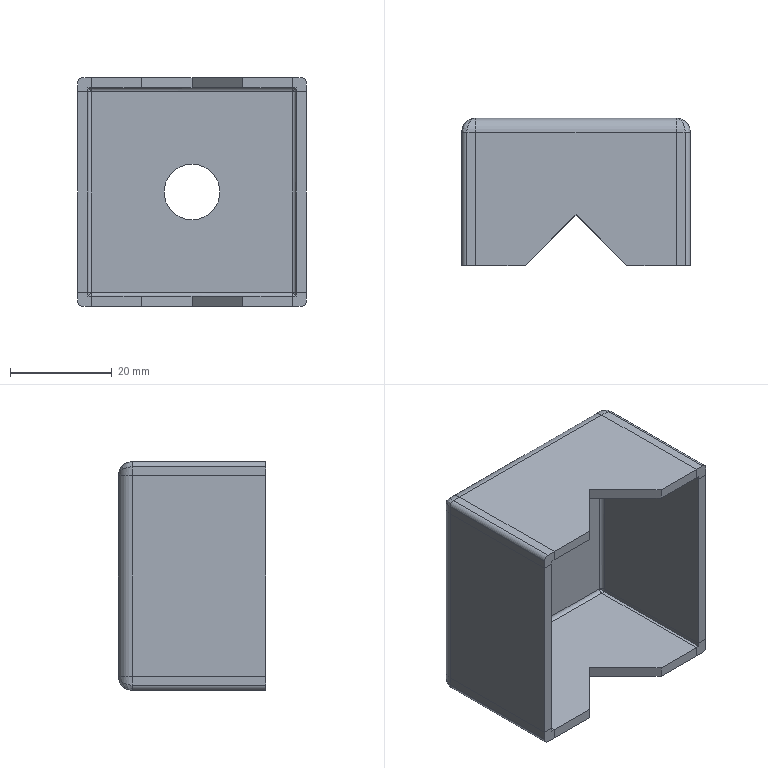Part | SolidWorks | features SMWeldBead 4, EdgeFlange 1, FlatPattern 1, ICE 1, SMBaseFlange 1, SheetMetal 1 | 1 solid | 74 faces | box 45 x 29 x 45 mm | volume 12461 mm3 | plane 40 | spline 20 | cylinder 14 | commonest cylinder face diameters 1.473 x4 2 x4 5.473 x4 11 x2